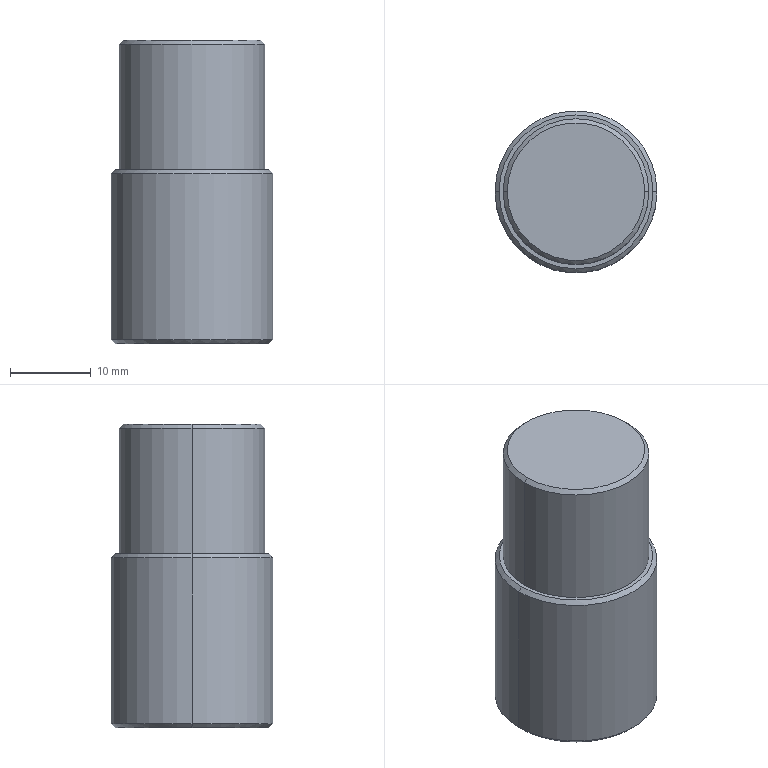Part | SolidWorks | features Chamfer 1, Extrusion 1, ICE 1 | 1 solid | 13 faces | box 20 x 20 x 37.5 mm | volume 10804 mm3 | cone 6 | cylinder 4 | plane 3 | commonest cylinder face diameters 18 x2 20 x2
STEP:
#1=CARTESIAN_POINT('',(9.5,0.,21.5));
#2=VERTEX_POINT('',#1);
#3=CARTESIAN_POINT('',(-9.5,0.,21.5));
#4=VERTEX_POINT('',#3);
#5=CARTESIAN_POINT('',(0.,0.,21.5));
#6=DIRECTION('',(0.,0.,1.));
#7=DIRECTION('',(-1.,0.,0.));
#8=AXIS2_PLACEMENT_3D('',#5,#6,#7);
#9=CIRCLE('',#8,9.5);
#10=EDGE_CURVE('',#2,#4,#9,.T.);
#11=ORIENTED_EDGE('',*,*,#10,.F.);
#12=CARTESIAN_POINT('',(10.,0.,21.));
#13=VERTEX_POINT('',#12);
#14=CARTESIAN_POINT('',(10.,0.,21.));
#15=DIRECTION('',(0.7071,0.,-0.7071));
#16=VECTOR('',#15,1000.);
#17=LINE('',#14,#16);
#18=EDGE_CURVE('',#2,#13,#17,.T.);
#19=ORIENTED_EDGE('',*,*,#18,.T.);
#20=CARTESIAN_POINT('',(-10.,0.,21.));
#21=VERTEX_POINT('',#20);
#22=CARTESIAN_POINT('',(0.,0.,21.));
#23=DIRECTION('',(0.,0.,-1.));
#24=DIRECTION('',(-1.,0.,0.));
#25=AXIS2_PLACEMENT_3D('',#22,#23,#24);
#26=CIRCLE('',#25,10.);
#27=EDGE_CURVE('',#21,#13,#26,.T.);
#28=ORIENTED_EDGE('',*,*,#27,.F.);
#29=CARTESIAN_POINT('',(-10.,0.,21.));
#30=DIRECTION('',(-0.7071,0.,-0.7071));
#31=VECTOR('',#30,1000.);
#32=LINE('',#29,#31);
#33=EDGE_CURVE('',#4,#21,#32,.T.);
#34=ORIENTED_EDGE('',*,*,#33,.F.);
#35=EDGE_LOOP('',(#11,#19,#28,#34));
#36=FACE_OUTER_BOUND('',#35,.T.);
#37=CARTESIAN_POINT('',(0.,0.,21.));
#38=DIRECTION('',(0.,0.,-1.));
#39=DIRECTION('',(-1.,0.,0.));
#40=AXIS2_PLACEMENT_3D('',#37,#38,#39);
#41=CONICAL_SURFACE('',#40,10.,0.7854);
#42=ADVANCED_FACE('',(#36),#41,.T.);
#43=CARTESIAN_POINT('',(-9.5,0.,0.));
#44=VERTEX_POINT('',#43);
#45=CARTESIAN_POINT('',(9.5,0.,0.));
#46=VERTEX_POINT('',#45);
#47=CARTESIAN_POINT('',(0.,0.,0.));
#48=DIRECTION('',(0.,0.,-1.));
#49=DIRECTION('',(1.,0.,0.));
#50=AXIS2_PLACEMENT_3D('',#47,#48,#49);
#51=CIRCLE('',#50,9.5);
#52=EDGE_CURVE('',#44,#46,#51,.T.);
#53=ORIENTED_EDGE('',*,*,#52,.F.);
#54=CARTESIAN_POINT('',(-10.,0.,0.5));
#55=VERTEX_POINT('',#54);
#56=CARTESIAN_POINT('',(-9.5,0.,0.));
#57=DIRECTION('',(-0.7071,0.,0.7071));
#58=VECTOR('',#57,1000.);
#59=LINE('',#56,#58);
#60=EDGE_CURVE('',#44,#55,#59,.T.);
#61=ORIENTED_EDGE('',*,*,#60,.T.);
#62=CARTESIAN_POINT('',(10.,0.,0.5));
#63=VERTEX_POINT('',#62);
#64=CARTESIAN_POINT('',(0.,0.,0.5));
#65=DIRECTION('',(0.,0.,1.));
#66=DIRECTION('',(1.,0.,0.));
#67=AXIS2_PLACEMENT_3D('',#64,#65,#66);
#68=CIRCLE('',#67,10.);
#69=EDGE_CURVE('',#63,#55,#68,.T.);
#70=ORIENTED_EDGE('',*,*,#69,.F.);
#71=CARTESIAN_POINT('',(9.5,0.,0.));
#72=DIRECTION('',(0.7071,0.,0.7071));
#73=VECTOR('',#72,1000.);
#74=LINE('',#71,#73);
#75=EDGE_CURVE('',#46,#63,#74,.T.);
#76=ORIENTED_EDGE('',*,*,#75,.F.);
#77=EDGE_LOOP('',(#53,#61,#70,#76));
#78=FACE_OUTER_BOUND('',#77,.T.);
#79=CARTESIAN_POINT('',(0.,0.,0.));
#80=DIRECTION('',(0.,0.,1.));
#81=DIRECTION('',(1.,0.,0.));
#82=AXIS2_PLACEMENT_3D('',#79,#80,#81);
#83=CONICAL_SURFACE('',#82,9.5,0.7854);
#84=ADVANCED_FACE('',(#78),#83,.T.);
#85=CARTESIAN_POINT('',(8.5,0.,37.5));
#86=VERTEX_POINT('',#85);
#87=CARTESIAN_POINT('',(-8.5,0.,37.5));
#88=VERTEX_POINT('',#87);
#89=CARTESIAN_POINT('',(0.,0.,37.5));
#90=DIRECTION('',(0.,0.,1.));
#91=DIRECTION('',(1.,0.,0.));
#92=AXIS2_PLACEMENT_3D('',#89,#90,#91);
#93=CIRCLE('',#92,8.5);
#94=EDGE_CURVE('',#86,#88,#93,.T.);
#95=ORIENTED_EDGE('',*,*,#94,.F.);
#96=CARTESIAN_POINT('',(9.,0.,37.));
#97=VERTEX_POINT('',#96);
#98=CARTESIAN_POINT('',(8.5,0.,37.5));
#99=DIRECTION('',(0.7071,0.,-0.7071));
#100=VECTOR('',#99,1000.);
#101=LINE('',#98,#100);
#102=EDGE_CURVE('',#86,#97,#101,.T.);
#103=ORIENTED_EDGE('',*,*,#102,.T.);
#104=CARTESIAN_POINT('',(-9.,0.,37.));
#105=VERTEX_POINT('',#104);
#106=CARTESIAN_POINT('',(0.,0.,37.));
#107=DIRECTION('',(0.,0.,-1.));
#108=DIRECTION('',(1.,0.,0.));
#109=AXIS2_PLACEMENT_3D('',#106,#107,#108);
#110=CIRCLE('',#109,9.);
#111=EDGE_CURVE('',#105,#97,#110,.T.);
#112=ORIENTED_EDGE('',*,*,#111,.F.);
#113=CARTESIAN_POINT('',(-8.5,0.,37.5));
#114=DIRECTION('',(-0.7071,0.,-0.7071));
#115=VECTOR('',#114,1000.);
#116=LINE('',#113,#115);
#117=EDGE_CURVE('',#88,#105,#116,.T.);
#118=ORIENTED_EDGE('',*,*,#117,.F.);
#119=EDGE_LOOP('',(#95,#103,#112,#118));
#120=FACE_OUTER_BOUND('',#119,.T.);
#121=CARTESIAN_POINT('',(0.,0.,37.5));
#122=DIRECTION('',(0.,0.,-1.));
#123=DIRECTION('',(-1.,0.,0.));
#124=AXIS2_PLACEMENT_3D('',#121,#122,#123);
#125=CONICAL_SURFACE('',#124,8.5,0.7854);
#126=ADVANCED_FACE('',(#120),#125,.T.);
#127=ORIENTED_EDGE('',*,*,#27,.T.);
#128=CARTESIAN_POINT('',(10.,0.,21.5));
#129=DIRECTION('',(0.,0.,-1.));
#130=VECTOR('',#129,1000.);
#131=LINE('',#128,#130);
#132=EDGE_CURVE('',#13,#63,#131,.T.);
#133=ORIENTED_EDGE('',*,*,#132,.T.);
#134=ORIENTED_EDGE('',*,*,#69,.T.);
#135=CARTESIAN_POINT('',(-10.,0.,21.5));
#136=DIRECTION('',(0.,0.,-1.));
#137=VECTOR('',#136,1000.);
#138=LINE('',#135,#137);
#139=EDGE_CURVE('',#21,#55,#138,.T.);
#140=ORIENTED_EDGE('',*,*,#139,.F.);
#141=EDGE_LOOP('',(#127,#133,#134,#140));
#142=FACE_OUTER_BOUND('',#141,.T.);
#143=CARTESIAN_POINT('',(0.,0.,21.5));
#144=DIRECTION('',(0.,0.,-1.));
#145=DIRECTION('',(-1.,0.,0.));
#146=AXIS2_PLACEMENT_3D('',#143,#144,#145);
#147=CYLINDRICAL_SURFACE('',#146,10.);
#148=ADVANCED_FACE('',(#142),#147,.T.);
#149=ORIENTED_EDGE('',*,*,#111,.T.);
#150=CARTESIAN_POINT('',(9.,0.,21.5));
#151=VERTEX_POINT('',#150);
#152=CARTESIAN_POINT('',(9.,0.,37.5));
#153=DIRECTION('',(0.,0.,-1.));
#154=VECTOR('',#153,1000.);
#155=LINE('',#152,#154);
#156=EDGE_CURVE('',#97,#151,#155,.T.);
#157=ORIENTED_EDGE('',*,*,#156,.T.);
#158=CARTESIAN_POINT('',(-9.,0.,21.5));
#159=VERTEX_POINT('',#158);
#160=CARTESIAN_POINT('',(0.,0.,21.5));
#161=DIRECTION('',(0.,0.,-1.));
#162=DIRECTION('',(-1.,0.,0.));
#163=AXIS2_PLACEMENT_3D('',#160,#161,#162);
#164=CIRCLE('',#163,9.);
#165=EDGE_CURVE('',#159,#151,#164,.T.);
#166=ORIENTED_EDGE('',*,*,#165,.F.);
#167=CARTESIAN_POINT('',(-9.,0.,37.5));
#168=DIRECTION('',(0.,0.,-1.));
#169=VECTOR('',#168,1000.);
#170=LINE('',#167,#169);
#171=EDGE_CURVE('',#105,#159,#170,.T.);
#172=ORIENTED_EDGE('',*,*,#171,.F.);
#173=EDGE_LOOP('',(#149,#157,#166,#172));
#174=FACE_OUTER_BOUND('',#173,.T.);
#175=CARTESIAN_POINT('',(0.,0.,37.5));
#176=DIRECTION('',(0.,0.,-1.));
#177=DIRECTION('',(-1.,0.,0.));
#178=AXIS2_PLACEMENT_3D('',#175,#176,#177);
#179=CYLINDRICAL_SURFACE('',#178,9.);
#180=ADVANCED_FACE('',(#174),#179,.T.);
#181=ORIENTED_EDGE('',*,*,#156,.F.);
#182=CARTESIAN_POINT('',(0.,0.,37.));
#183=DIRECTION('',(0.,0.,-1.));
#184=DIRECTION('',(1.,0.,0.));
#185=AXIS2_PLACEMENT_3D('',#182,#183,#184);
#186=CIRCLE('',#185,9.);
#187=EDGE_CURVE('',#97,#105,#186,.T.);
#188=ORIENTED_EDGE('',*,*,#187,.T.);
#189=ORIENTED_EDGE('',*,*,#171,.T.);
#190=CARTESIAN_POINT('',(0.,0.,21.5));
#191=DIRECTION('',(0.,0.,-1.));
#192=DIRECTION('',(-1.,0.,0.));
#193=AXIS2_PLACEMENT_3D('',#190,#191,#192);
#194=CIRCLE('',#193,9.);
#195=EDGE_CURVE('',#151,#159,#194,.T.);
#196=ORIENTED_EDGE('',*,*,#195,.F.);
#197=EDGE_LOOP('',(#181,#188,#189,#196));
#198=FACE_OUTER_BOUND('',#197,.T.);
#199=CARTESIAN_POINT('',(0.,0.,37.5));
#200=DIRECTION('',(0.,0.,-1.));
#201=DIRECTION('',(-1.,0.,0.));
#202=AXIS2_PLACEMENT_3D('',#199,#200,#201);
#203=CYLINDRICAL_SURFACE('',#202,9.);
#204=ADVANCED_FACE('',(#198),#203,.T.);
#205=CARTESIAN_POINT('',(0.,0.,37.5));
#206=DIRECTION('',(0.,0.,1.));
#207=DIRECTION('',(1.,0.,0.));
#208=AXIS2_PLACEMENT_3D('',#205,#206,#207);
#209=CIRCLE('',#208,8.5);
#210=EDGE_CURVE('',#88,#86,#209,.T.);
#211=ORIENTED_EDGE('',*,*,#210,.T.);
#212=ORIENTED_EDGE('',*,*,#94,.T.);
#213=EDGE_LOOP('',(#211,#212));
#214=FACE_OUTER_BOUND('',#213,.T.);
#215=CARTESIAN_POINT('',(0.,0.,37.5));
#216=DIRECTION('',(0.,0.,1.));
#217=DIRECTION('',(1.,0.,0.));
#218=AXIS2_PLACEMENT_3D('',#215,#216,#217);
#219=PLANE('',#218);
#220=ADVANCED_FACE('',(#214),#219,.T.);
#221=ORIENTED_EDGE('',*,*,#132,.F.);
#222=CARTESIAN_POINT('',(0.,0.,21.));
#223=DIRECTION('',(0.,0.,-1.));
#224=DIRECTION('',(-1.,0.,0.));
#225=AXIS2_PLACEMENT_3D('',#222,#223,#224);
#226=CIRCLE('',#225,10.);
#227=EDGE_CURVE('',#13,#21,#226,.T.);
#228=ORIENTED_EDGE('',*,*,#227,.T.);
#229=ORIENTED_EDGE('',*,*,#139,.T.);
#230=CARTESIAN_POINT('',(0.,0.,0.5));
#231=DIRECTION('',(0.,0.,1.));
#232=DIRECTION('',(1.,0.,0.));
#233=AXIS2_PLACEMENT_3D('',#230,#231,#232);
#234=CIRCLE('',#233,10.);
#235=EDGE_CURVE('',#55,#63,#234,.T.);
#236=ORIENTED_EDGE('',*,*,#235,.T.);
#237=EDGE_LOOP('',(#221,#228,#229,#236));
#238=FACE_OUTER_BOUND('',#237,.T.);
#239=CARTESIAN_POINT('',(0.,0.,21.5));
#240=DIRECTION('',(0.,0.,-1.));
#241=DIRECTION('',(-1.,0.,0.));
#242=AXIS2_PLACEMENT_3D('',#239,#240,#241);
#243=CYLINDRICAL_SURFACE('',#242,10.);
#244=ADVANCED_FACE('',(#238),#243,.T.);
#245=CARTESIAN_POINT('',(0.,0.,21.5));
#246=DIRECTION('',(0.,0.,1.));
#247=DIRECTION('',(-1.,0.,0.));
#248=AXIS2_PLACEMENT_3D('',#245,#246,#247);
#249=CIRCLE('',#248,9.5);
#250=EDGE_CURVE('',#4,#2,#249,.T.);
#251=ORIENTED_EDGE('',*,*,#250,.T.);
#252=ORIENTED_EDGE('',*,*,#10,.T.);
#253=EDGE_LOOP('',(#251,#252));
#254=FACE_OUTER_BOUND('',#253,.T.);
#255=ORIENTED_EDGE('',*,*,#165,.T.);
#256=ORIENTED_EDGE('',*,*,#195,.T.);
#257=EDGE_LOOP('',(#255,#256));
#258=FACE_BOUND('',#257,.T.);
#259=CARTESIAN_POINT('',(0.,0.,21.5));
#260=DIRECTION('',(0.,0.,-1.));
#261=DIRECTION('',(-1.,0.,0.));
#262=AXIS2_PLACEMENT_3D('',#259,#260,#261);
#263=PLANE('',#262);
#264=ADVANCED_FACE('',(#254,#258),#263,.F.);
#265=CARTESIAN_POINT('',(0.,0.,0.));
#266=DIRECTION('',(0.,0.,-1.));
#267=DIRECTION('',(1.,0.,0.));
#268=AXIS2_PLACEMENT_3D('',#265,#266,#267);
#269=CIRCLE('',#268,9.5);
#270=EDGE_CURVE('',#46,#44,#269,.T.);
#271=ORIENTED_EDGE('',*,*,#270,.T.);
#272=ORIENTED_EDGE('',*,*,#52,.T.);
#273=EDGE_LOOP('',(#271,#272));
#274=FACE_OUTER_BOUND('',#273,.T.);
#275=CARTESIAN_POINT('',(0.,0.,0.));
#276=DIRECTION('',(0.,0.,1.));
#277=DIRECTION('',(1.,0.,0.));
#278=AXIS2_PLACEMENT_3D('',#275,#276,#277);
#279=PLANE('',#278);
#280=ADVANCED_FACE('',(#274),#279,.F.);
#281=ORIENTED_EDGE('',*,*,#102,.F.);
#282=ORIENTED_EDGE('',*,*,#210,.F.);
#283=ORIENTED_EDGE('',*,*,#117,.T.);
#284=ORIENTED_EDGE('',*,*,#187,.F.);
#285=EDGE_LOOP('',(#281,#282,#283,#284));
#286=FACE_OUTER_BOUND('',#285,.T.);
#287=CARTESIAN_POINT('',(0.,0.,37.5));
#288=DIRECTION('',(0.,0.,-1.));
#289=DIRECTION('',(-1.,0.,0.));
#290=AXIS2_PLACEMENT_3D('',#287,#288,#289);
#291=CONICAL_SURFACE('',#290,8.5,0.7854);
#292=ADVANCED_FACE('',(#286),#291,.T.);
#293=ORIENTED_EDGE('',*,*,#60,.F.);
#294=ORIENTED_EDGE('',*,*,#270,.F.);
#295=ORIENTED_EDGE('',*,*,#75,.T.);
#296=ORIENTED_EDGE('',*,*,#235,.F.);
#297=EDGE_LOOP('',(#293,#294,#295,#296));
#298=FACE_OUTER_BOUND('',#297,.T.);
#299=CARTESIAN_POINT('',(0.,0.,0.));
#300=DIRECTION('',(0.,0.,1.));
#301=DIRECTION('',(1.,0.,0.));
#302=AXIS2_PLACEMENT_3D('',#299,#300,#301);
#303=CONICAL_SURFACE('',#302,9.5,0.7854);
#304=ADVANCED_FACE('',(#298),#303,.T.);
#305=ORIENTED_EDGE('',*,*,#18,.F.);
#306=ORIENTED_EDGE('',*,*,#250,.F.);
#307=ORIENTED_EDGE('',*,*,#33,.T.);
#308=ORIENTED_EDGE('',*,*,#227,.F.);
#309=EDGE_LOOP('',(#305,#306,#307,#308));
#310=FACE_OUTER_BOUND('',#309,.T.);
#311=CARTESIAN_POINT('',(0.,0.,21.));
#312=DIRECTION('',(0.,0.,-1.));
#313=DIRECTION('',(-1.,0.,0.));
#314=AXIS2_PLACEMENT_3D('',#311,#312,#313);
#315=CONICAL_SURFACE('',#314,10.,0.7854);
#316=ADVANCED_FACE('',(#310),#315,.T.);
#317=CLOSED_SHELL('',(#42,#84,#126,#148,#180,#204,#220,#244,#264,#280,#292,#304,#316));
#318=MANIFOLD_SOLID_BREP('',#317);
#319=CARTESIAN_POINT('',(0.,0.,0.));
#320=DIRECTION('',(0.,0.,1.));
#321=DIRECTION('',(1.,0.,0.));
#322=AXIS2_PLACEMENT_3D('',#319,#320,#321);
#323=(LENGTH_UNIT()NAMED_UNIT(*)SI_UNIT(.MILLI.,.METRE.));
#324=UNCERTAINTY_MEASURE_WITH_UNIT(LENGTH_MEASURE(0.00001),#323,'','');
#325=(NAMED_UNIT(*)PLANE_ANGLE_UNIT()SI_UNIT($,.RADIAN.));
#326=(NAMED_UNIT(*)SI_UNIT($,.STERADIAN.)SOLID_ANGLE_UNIT());
#327=(GEOMETRIC_REPRESENTATION_CONTEXT(3)GLOBAL_UNCERTAINTY_ASSIGNED_CONTEXT((#324))GLOBAL_UNIT_ASSIGNED_CONTEXT((#323,#325,#326))REPRESENTATION_CONTEXT('',''));
#328=ADVANCED_BREP_SHAPE_REPRESENTATION('',(#318,#322),#327);